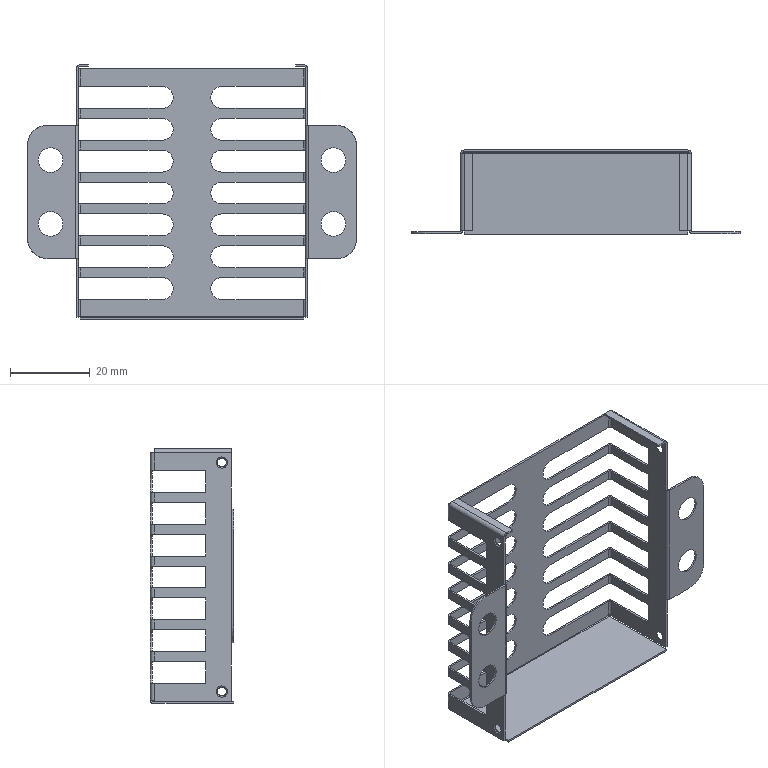Part | NX | features BREP 1 | 1 solid | 236 faces | box 82.56 x 21 x 63.94 mm | volume 2450 mm3 | plane 152 | cylinder 76 | cone 8 | commonest cylinder face diameters 1 x18 1.94 x18 5.5 x14 2.2 x8 6.2 x8 10 x4